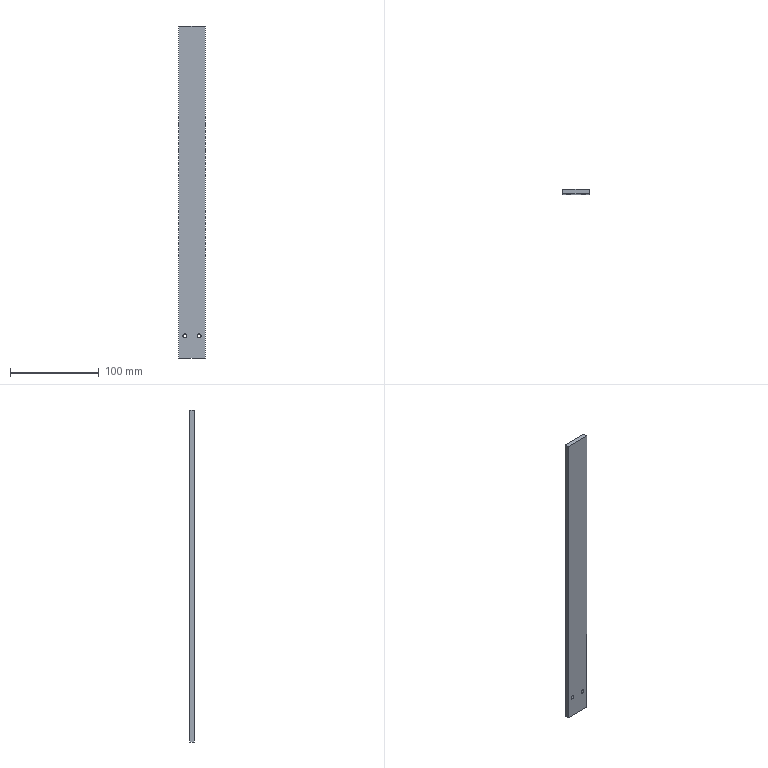Part | SolidWorks | features ICE 4, Cut 1, Extrusion 1, MirrorSolid 1 | 1 solid | 10 faces | box 30 x 5 x 375 mm | volume 56098 mm3 | plane 6 | cylinder 4 | commonest cylinder face diameters 4.4 x4
STEP:
#1=CARTESIAN_POINT('',(8.,-5.,-337.2));
#2=VERTEX_POINT('',#1);
#3=CARTESIAN_POINT('',(8.,-5.,-332.8));
#4=VERTEX_POINT('',#3);
#5=CARTESIAN_POINT('',(8.,-5.,-335.));
#6=DIRECTION('',(0.,1.,0.));
#7=DIRECTION('',(0.,0.,1.));
#8=AXIS2_PLACEMENT_3D('',#5,#6,#7);
#9=CIRCLE('',#8,2.2);
#10=EDGE_CURVE('',#2,#4,#9,.T.);
#11=ORIENTED_EDGE('',*,*,#10,.F.);
#12=CARTESIAN_POINT('',(8.,0.,-337.2));
#13=VERTEX_POINT('',#12);
#14=CARTESIAN_POINT('',(8.,-5.,-337.2));
#15=DIRECTION('',(0.,1.,0.));
#16=VECTOR('',#15,1000.);
#17=LINE('',#14,#16);
#18=EDGE_CURVE('',#2,#13,#17,.T.);
#19=ORIENTED_EDGE('',*,*,#18,.T.);
#20=CARTESIAN_POINT('',(8.,0.,-332.8));
#21=VERTEX_POINT('',#20);
#22=CARTESIAN_POINT('',(8.,0.,-335.));
#23=DIRECTION('',(0.,-1.,0.));
#24=DIRECTION('',(0.,0.,1.));
#25=AXIS2_PLACEMENT_3D('',#22,#23,#24);
#26=CIRCLE('',#25,2.2);
#27=EDGE_CURVE('',#21,#13,#26,.T.);
#28=ORIENTED_EDGE('',*,*,#27,.F.);
#29=CARTESIAN_POINT('',(8.,-5.,-332.8));
#30=DIRECTION('',(0.,1.,0.));
#31=VECTOR('',#30,1000.);
#32=LINE('',#29,#31);
#33=EDGE_CURVE('',#4,#21,#32,.T.);
#34=ORIENTED_EDGE('',*,*,#33,.F.);
#35=EDGE_LOOP('',(#11,#19,#28,#34));
#36=FACE_OUTER_BOUND('',#35,.T.);
#37=CARTESIAN_POINT('',(8.,-5.,-335.));
#38=DIRECTION('',(0.,1.,0.));
#39=DIRECTION('',(0.,0.,1.));
#40=AXIS2_PLACEMENT_3D('',#37,#38,#39);
#41=CYLINDRICAL_SURFACE('',#40,2.2);
#42=ADVANCED_FACE('',(#36),#41,.F.);
#43=CARTESIAN_POINT('',(-8.,-5.,-337.2));
#44=VERTEX_POINT('',#43);
#45=CARTESIAN_POINT('',(-8.,-5.,-332.8));
#46=VERTEX_POINT('',#45);
#47=CARTESIAN_POINT('',(-8.,-5.,-335.));
#48=DIRECTION('',(0.,1.,0.));
#49=DIRECTION('',(0.,0.,1.));
#50=AXIS2_PLACEMENT_3D('',#47,#48,#49);
#51=CIRCLE('',#50,2.2);
#52=EDGE_CURVE('',#44,#46,#51,.T.);
#53=ORIENTED_EDGE('',*,*,#52,.F.);
#54=CARTESIAN_POINT('',(-8.,0.,-337.2));
#55=VERTEX_POINT('',#54);
#56=CARTESIAN_POINT('',(-8.,-5.,-337.2));
#57=DIRECTION('',(0.,1.,0.));
#58=VECTOR('',#57,1000.);
#59=LINE('',#56,#58);
#60=EDGE_CURVE('',#44,#55,#59,.T.);
#61=ORIENTED_EDGE('',*,*,#60,.T.);
#62=CARTESIAN_POINT('',(-8.,0.,-332.8));
#63=VERTEX_POINT('',#62);
#64=CARTESIAN_POINT('',(-8.,0.,-335.));
#65=DIRECTION('',(0.,-1.,0.));
#66=DIRECTION('',(0.,0.,1.));
#67=AXIS2_PLACEMENT_3D('',#64,#65,#66);
#68=CIRCLE('',#67,2.2);
#69=EDGE_CURVE('',#63,#55,#68,.T.);
#70=ORIENTED_EDGE('',*,*,#69,.F.);
#71=CARTESIAN_POINT('',(-8.,-5.,-332.8));
#72=DIRECTION('',(0.,1.,0.));
#73=VECTOR('',#72,1000.);
#74=LINE('',#71,#73);
#75=EDGE_CURVE('',#46,#63,#74,.T.);
#76=ORIENTED_EDGE('',*,*,#75,.F.);
#77=EDGE_LOOP('',(#53,#61,#70,#76));
#78=FACE_OUTER_BOUND('',#77,.T.);
#79=CARTESIAN_POINT('',(-8.,-5.,-335.));
#80=DIRECTION('',(0.,1.,0.));
#81=DIRECTION('',(0.,0.,1.));
#82=AXIS2_PLACEMENT_3D('',#79,#80,#81);
#83=CYLINDRICAL_SURFACE('',#82,2.2);
#84=ADVANCED_FACE('',(#78),#83,.F.);
#85=CARTESIAN_POINT('',(-15.,0.,-360.));
#86=VERTEX_POINT('',#85);
#87=CARTESIAN_POINT('',(-15.,0.,15.));
#88=VERTEX_POINT('',#87);
#89=CARTESIAN_POINT('',(-15.,0.,-360.));
#90=DIRECTION('',(0.,0.,1.));
#91=VECTOR('',#90,1000.);
#92=LINE('',#89,#91);
#93=EDGE_CURVE('',#86,#88,#92,.T.);
#94=ORIENTED_EDGE('',*,*,#93,.F.);
#95=CARTESIAN_POINT('',(-15.,-5.,-360.));
#96=VERTEX_POINT('',#95);
#97=CARTESIAN_POINT('',(-15.,-2.5,-360.));
#98=DIRECTION('',(0.,-1.,0.));
#99=VECTOR('',#98,1000.);
#100=LINE('',#97,#99);
#101=EDGE_CURVE('',#86,#96,#100,.T.);
#102=ORIENTED_EDGE('',*,*,#101,.T.);
#103=CARTESIAN_POINT('',(-15.,-5.,15.));
#104=VERTEX_POINT('',#103);
#105=CARTESIAN_POINT('',(-15.,-5.,-172.5));
#106=DIRECTION('',(0.,0.,1.));
#107=VECTOR('',#106,1000.);
#108=LINE('',#105,#107);
#109=EDGE_CURVE('',#96,#104,#108,.T.);
#110=ORIENTED_EDGE('',*,*,#109,.T.);
#111=CARTESIAN_POINT('',(-15.,-2.5,15.));
#112=DIRECTION('',(0.,-1.,0.));
#113=VECTOR('',#112,1000.);
#114=LINE('',#111,#113);
#115=EDGE_CURVE('',#88,#104,#114,.T.);
#116=ORIENTED_EDGE('',*,*,#115,.F.);
#117=EDGE_LOOP('',(#94,#102,#110,#116));
#118=FACE_OUTER_BOUND('',#117,.T.);
#119=CARTESIAN_POINT('',(-15.,-2.5,15.));
#120=DIRECTION('',(1.,0.,0.));
#121=DIRECTION('',(0.,0.,-1.));
#122=AXIS2_PLACEMENT_3D('',#119,#120,#121);
#123=PLANE('',#122);
#124=ADVANCED_FACE('',(#118),#123,.F.);
#125=CARTESIAN_POINT('',(15.,0.,15.));
#126=VERTEX_POINT('',#125);
#127=CARTESIAN_POINT('',(15.,0.,-360.));
#128=VERTEX_POINT('',#127);
#129=CARTESIAN_POINT('',(15.,0.,15.));
#130=DIRECTION('',(0.,0.,-1.));
#131=VECTOR('',#130,1000.);
#132=LINE('',#129,#131);
#133=EDGE_CURVE('',#126,#128,#132,.T.);
#134=ORIENTED_EDGE('',*,*,#133,.F.);
#135=CARTESIAN_POINT('',(15.,-5.,15.));
#136=VERTEX_POINT('',#135);
#137=CARTESIAN_POINT('',(15.,-2.5,15.));
#138=DIRECTION('',(0.,1.,0.));
#139=VECTOR('',#138,1000.);
#140=LINE('',#137,#139);
#141=EDGE_CURVE('',#136,#126,#140,.T.);
#142=ORIENTED_EDGE('',*,*,#141,.F.);
#143=CARTESIAN_POINT('',(15.,-5.,-360.));
#144=VERTEX_POINT('',#143);
#145=CARTESIAN_POINT('',(15.,-5.,-172.5));
#146=DIRECTION('',(0.,0.,1.));
#147=VECTOR('',#146,1000.);
#148=LINE('',#145,#147);
#149=EDGE_CURVE('',#144,#136,#148,.T.);
#150=ORIENTED_EDGE('',*,*,#149,.F.);
#151=CARTESIAN_POINT('',(15.,-2.5,-360.));
#152=DIRECTION('',(0.,1.,0.));
#153=VECTOR('',#152,1000.);
#154=LINE('',#151,#153);
#155=EDGE_CURVE('',#144,#128,#154,.T.);
#156=ORIENTED_EDGE('',*,*,#155,.T.);
#157=EDGE_LOOP('',(#134,#142,#150,#156));
#158=FACE_OUTER_BOUND('',#157,.T.);
#159=CARTESIAN_POINT('',(15.,-2.5,15.));
#160=DIRECTION('',(-1.,0.,0.));
#161=DIRECTION('',(0.,0.,1.));
#162=AXIS2_PLACEMENT_3D('',#159,#160,#161);
#163=PLANE('',#162);
#164=ADVANCED_FACE('',(#158),#163,.F.);
#165=ORIENTED_EDGE('',*,*,#141,.T.);
#166=CARTESIAN_POINT('',(-15.,0.,15.));
#167=DIRECTION('',(1.,0.,0.));
#168=VECTOR('',#167,1000.);
#169=LINE('',#166,#168);
#170=EDGE_CURVE('',#88,#126,#169,.T.);
#171=ORIENTED_EDGE('',*,*,#170,.F.);
#172=ORIENTED_EDGE('',*,*,#115,.T.);
#173=CARTESIAN_POINT('',(-15.,-5.,15.));
#174=DIRECTION('',(1.,0.,0.));
#175=VECTOR('',#174,1000.);
#176=LINE('',#173,#175);
#177=EDGE_CURVE('',#104,#136,#176,.T.);
#178=ORIENTED_EDGE('',*,*,#177,.T.);
#179=EDGE_LOOP('',(#165,#171,#172,#178));
#180=FACE_OUTER_BOUND('',#179,.T.);
#181=CARTESIAN_POINT('',(0.,0.,15.));
#182=DIRECTION('',(0.,0.,1.));
#183=DIRECTION('',(1.,0.,0.));
#184=AXIS2_PLACEMENT_3D('',#181,#182,#183);
#185=PLANE('',#184);
#186=ADVANCED_FACE('',(#180),#185,.T.);
#187=ORIENTED_EDGE('',*,*,#101,.F.);
#188=CARTESIAN_POINT('',(15.,0.,-360.));
#189=DIRECTION('',(-1.,0.,0.));
#190=VECTOR('',#189,1000.);
#191=LINE('',#188,#190);
#192=EDGE_CURVE('',#128,#86,#191,.T.);
#193=ORIENTED_EDGE('',*,*,#192,.F.);
#194=ORIENTED_EDGE('',*,*,#155,.F.);
#195=CARTESIAN_POINT('',(15.,-5.,-360.));
#196=DIRECTION('',(-1.,0.,0.));
#197=VECTOR('',#196,1000.);
#198=LINE('',#195,#197);
#199=EDGE_CURVE('',#144,#96,#198,.T.);
#200=ORIENTED_EDGE('',*,*,#199,.T.);
#201=EDGE_LOOP('',(#187,#193,#194,#200));
#202=FACE_OUTER_BOUND('',#201,.T.);
#203=CARTESIAN_POINT('',(0.,0.,-360.));
#204=DIRECTION('',(0.,0.,-1.));
#205=DIRECTION('',(1.,0.,0.));
#206=AXIS2_PLACEMENT_3D('',#203,#204,#205);
#207=PLANE('',#206);
#208=ADVANCED_FACE('',(#202),#207,.T.);
#209=ORIENTED_EDGE('',*,*,#60,.F.);
#210=CARTESIAN_POINT('',(-8.,-5.,-335.));
#211=DIRECTION('',(0.,1.,0.));
#212=DIRECTION('',(0.,0.,1.));
#213=AXIS2_PLACEMENT_3D('',#210,#211,#212);
#214=CIRCLE('',#213,2.2);
#215=EDGE_CURVE('',#46,#44,#214,.T.);
#216=ORIENTED_EDGE('',*,*,#215,.F.);
#217=ORIENTED_EDGE('',*,*,#75,.T.);
#218=CARTESIAN_POINT('',(-8.,0.,-335.));
#219=DIRECTION('',(0.,-1.,0.));
#220=DIRECTION('',(0.,0.,1.));
#221=AXIS2_PLACEMENT_3D('',#218,#219,#220);
#222=CIRCLE('',#221,2.2);
#223=EDGE_CURVE('',#55,#63,#222,.T.);
#224=ORIENTED_EDGE('',*,*,#223,.F.);
#225=EDGE_LOOP('',(#209,#216,#217,#224));
#226=FACE_OUTER_BOUND('',#225,.T.);
#227=CARTESIAN_POINT('',(-8.,-5.,-335.));
#228=DIRECTION('',(0.,1.,0.));
#229=DIRECTION('',(0.,0.,1.));
#230=AXIS2_PLACEMENT_3D('',#227,#228,#229);
#231=CYLINDRICAL_SURFACE('',#230,2.2);
#232=ADVANCED_FACE('',(#226),#231,.F.);
#233=ORIENTED_EDGE('',*,*,#18,.F.);
#234=CARTESIAN_POINT('',(8.,-5.,-335.));
#235=DIRECTION('',(0.,1.,0.));
#236=DIRECTION('',(0.,0.,1.));
#237=AXIS2_PLACEMENT_3D('',#234,#235,#236);
#238=CIRCLE('',#237,2.2);
#239=EDGE_CURVE('',#4,#2,#238,.T.);
#240=ORIENTED_EDGE('',*,*,#239,.F.);
#241=ORIENTED_EDGE('',*,*,#33,.T.);
#242=CARTESIAN_POINT('',(8.,0.,-335.));
#243=DIRECTION('',(0.,-1.,0.));
#244=DIRECTION('',(0.,0.,1.));
#245=AXIS2_PLACEMENT_3D('',#242,#243,#244);
#246=CIRCLE('',#245,2.2);
#247=EDGE_CURVE('',#13,#21,#246,.T.);
#248=ORIENTED_EDGE('',*,*,#247,.F.);
#249=EDGE_LOOP('',(#233,#240,#241,#248));
#250=FACE_OUTER_BOUND('',#249,.T.);
#251=CARTESIAN_POINT('',(8.,-5.,-335.));
#252=DIRECTION('',(0.,1.,0.));
#253=DIRECTION('',(0.,0.,1.));
#254=AXIS2_PLACEMENT_3D('',#251,#252,#253);
#255=CYLINDRICAL_SURFACE('',#254,2.2);
#256=ADVANCED_FACE('',(#250),#255,.F.);
#257=ORIENTED_EDGE('',*,*,#239,.T.);
#258=ORIENTED_EDGE('',*,*,#10,.T.);
#259=EDGE_LOOP('',(#257,#258));
#260=FACE_BOUND('',#259,.T.);
#261=ORIENTED_EDGE('',*,*,#215,.T.);
#262=ORIENTED_EDGE('',*,*,#52,.T.);
#263=EDGE_LOOP('',(#261,#262));
#264=FACE_BOUND('',#263,.T.);
#265=ORIENTED_EDGE('',*,*,#149,.T.);
#266=ORIENTED_EDGE('',*,*,#177,.F.);
#267=ORIENTED_EDGE('',*,*,#109,.F.);
#268=ORIENTED_EDGE('',*,*,#199,.F.);
#269=EDGE_LOOP('',(#265,#266,#267,#268));
#270=FACE_OUTER_BOUND('',#269,.T.);
#271=CARTESIAN_POINT('',(-15.,-5.,-172.5));
#272=DIRECTION('',(0.,1.,0.));
#273=DIRECTION('',(0.,0.,1.));
#274=AXIS2_PLACEMENT_3D('',#271,#272,#273);
#275=PLANE('',#274);
#276=ADVANCED_FACE('',(#260,#264,#270),#275,.F.);
#277=ORIENTED_EDGE('',*,*,#192,.T.);
#278=ORIENTED_EDGE('',*,*,#93,.T.);
#279=ORIENTED_EDGE('',*,*,#170,.T.);
#280=ORIENTED_EDGE('',*,*,#133,.T.);
#281=EDGE_LOOP('',(#277,#278,#279,#280));
#282=FACE_OUTER_BOUND('',#281,.T.);
#283=ORIENTED_EDGE('',*,*,#27,.T.);
#284=ORIENTED_EDGE('',*,*,#247,.T.);
#285=EDGE_LOOP('',(#283,#284));
#286=FACE_BOUND('',#285,.T.);
#287=ORIENTED_EDGE('',*,*,#69,.T.);
#288=ORIENTED_EDGE('',*,*,#223,.T.);
#289=EDGE_LOOP('',(#287,#288));
#290=FACE_BOUND('',#289,.T.);
#291=CARTESIAN_POINT('',(0.,0.,0.));
#292=DIRECTION('',(0.,1.,0.));
#293=DIRECTION('',(0.,0.,1.));
#294=AXIS2_PLACEMENT_3D('',#291,#292,#293);
#295=PLANE('',#294);
#296=ADVANCED_FACE('',(#282,#286,#290),#295,.T.);
#297=CLOSED_SHELL('',(#42,#84,#124,#164,#186,#208,#232,#256,#276,#296));
#298=MANIFOLD_SOLID_BREP('',#297);
#299=CARTESIAN_POINT('',(0.,0.,0.));
#300=DIRECTION('',(0.,0.,1.));
#301=DIRECTION('',(1.,0.,0.));
#302=AXIS2_PLACEMENT_3D('',#299,#300,#301);
#303=(LENGTH_UNIT()NAMED_UNIT(*)SI_UNIT(.MILLI.,.METRE.));
#304=UNCERTAINTY_MEASURE_WITH_UNIT(LENGTH_MEASURE(0.00001),#303,'','');
#305=(NAMED_UNIT(*)PLANE_ANGLE_UNIT()SI_UNIT($,.RADIAN.));
#306=(NAMED_UNIT(*)SI_UNIT($,.STERADIAN.)SOLID_ANGLE_UNIT());
#307=(GEOMETRIC_REPRESENTATION_CONTEXT(3)GLOBAL_UNCERTAINTY_ASSIGNED_CONTEXT((#304))GLOBAL_UNIT_ASSIGNED_CONTEXT((#303,#305,#306))REPRESENTATION_CONTEXT('',''));
#308=ADVANCED_BREP_SHAPE_REPRESENTATION('',(#298,#302),#307);